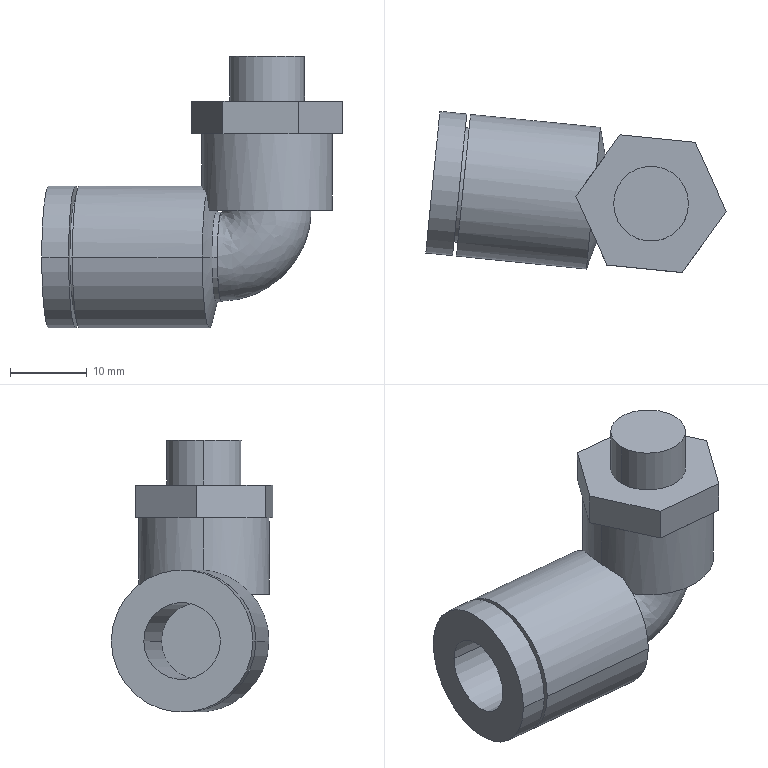Part | SolidWorks | features BaseBody 1 | 1 solid | 38 faces | box 39.045 x 20.983 x 35.35 mm | volume 8720 mm3 | plane 20 | cylinder 14 | cone 2 | spline 2 | commonest cylinder face diameters 18.5 x4 9.728 x2 10 x2 11.729 x2 15 x2 17 x2
STEP:
#1=CARTESIAN_POINT('',(-83.459,11.64,316.618));
#2=VERTEX_POINT('',#1);
#3=CARTESIAN_POINT('',(-85.298,-6.769,316.618));
#4=VERTEX_POINT('',#3);
#5=CARTESIAN_POINT('',(-84.379,2.436,316.618));
#6=DIRECTION('',(0.995,-0.09941,0.));
#7=DIRECTION('',(0.09941,0.995,0.));
#8=AXIS2_PLACEMENT_3D('',#5,#6,#7);
#9=CIRCLE('',#8,9.25);
#10=EDGE_CURVE('',#2,#4,#9,.T.);
#11=ORIENTED_EDGE('',*,*,#10,.T.);
#12=CARTESIAN_POINT('',(-68.414,-8.455,316.618));
#13=VERTEX_POINT('',#12);
#14=CARTESIAN_POINT('',(-76.856,-7.612,316.618));
#15=DIRECTION('',(0.995,-0.09941,0.));
#16=VECTOR('',#15,1000.);
#17=LINE('',#14,#16);
#18=EDGE_CURVE('',#4,#13,#17,.T.);
#19=ORIENTED_EDGE('',*,*,#18,.T.);
#20=CARTESIAN_POINT('',(-67.886,-3.171,324.987));
#21=VERTEX_POINT('',#20);
#22=CARTESIAN_POINT('',(-67.495,0.7488,316.618));
#23=DIRECTION('',(-0.995,0.09941,0.));
#24=DIRECTION('',(0.09941,0.995,0.));
#25=AXIS2_PLACEMENT_3D('',#22,#23,#24);
#26=CIRCLE('',#25,9.25);
#27=EDGE_CURVE('',#13,#21,#26,.T.);
#28=ORIENTED_EDGE('',*,*,#27,.T.);
#29=CARTESIAN_POINT('',(-68.5,0.,325.829));
#30=VERTEX_POINT('',#29);
#31=CARTESIAN_POINT('',(-67.886,-3.171,324.987));
#32=CARTESIAN_POINT('',(-68.081,-2.687,325.205));
#33=CARTESIAN_POINT('',(-68.233,-2.18,325.388));
#34=CARTESIAN_POINT('',(-68.391,-1.383,325.604));
#35=CARTESIAN_POINT('',(-68.432,-1.11,325.666));
#36=CARTESIAN_POINT('',(-68.486,-0.5568,325.766));
#37=CARTESIAN_POINT('',(-68.5,-0.2791,325.804));
#38=CARTESIAN_POINT('',(-68.5,0.,325.829));
#39=B_SPLINE_CURVE_WITH_KNOTS('',3,(#31,#32,#33,#34,#35,#36,#37,#38),.UNSPECIFIED.,.F.,.F.,(4,2,2,4),(-0.004184,-0.002512,-0.001676,-0.0008395),.UNSPECIFIED.);
#40=EDGE_CURVE('',#21,#30,#39,.T.);
#41=ORIENTED_EDGE('',*,*,#40,.T.);
#42=CARTESIAN_POINT('',(-67.103,4.668,324.987));
#43=VERTEX_POINT('',#42);
#44=CARTESIAN_POINT('',(-68.5,0.,325.829));
#45=CARTESIAN_POINT('',(-68.5,0.2097,325.848));
#46=CARTESIAN_POINT('',(-68.492,0.4202,325.86));
#47=CARTESIAN_POINT('',(-68.461,0.8429,325.87));
#48=CARTESIAN_POINT('',(-68.437,1.055,325.868));
#49=CARTESIAN_POINT('',(-68.343,1.68,325.839));
#50=CARTESIAN_POINT('',(-68.251,2.086,325.792));
#51=CARTESIAN_POINT('',(-68.009,2.877,325.643));
#52=CARTESIAN_POINT('',(-67.858,3.265,325.542));
#53=CARTESIAN_POINT('',(-67.513,3.995,325.295));
#54=CARTESIAN_POINT('',(-67.319,4.341,325.151));
#55=CARTESIAN_POINT('',(-67.103,4.668,324.987));
#56=B_SPLINE_CURVE_WITH_KNOTS('',3,(#44,#45,#46,#47,#48,#49,#50,#51,#52,#53,#54,#55),.UNSPECIFIED.,.F.,.F.,(4,2,2,2,2,4),(-0.0008395,-0.0002113,0.000417,0.001674,0.00293,0.004187),.UNSPECIFIED.);
#57=EDGE_CURVE('',#30,#43,#56,.T.);
#58=ORIENTED_EDGE('',*,*,#57,.T.);
#59=CARTESIAN_POINT('',(-66.575,9.953,316.618));
#60=VERTEX_POINT('',#59);
#61=CARTESIAN_POINT('',(-67.495,0.7488,316.618));
#62=DIRECTION('',(-0.995,0.09941,0.));
#63=DIRECTION('',(0.09941,0.995,0.));
#64=AXIS2_PLACEMENT_3D('',#61,#62,#63);
#65=CIRCLE('',#64,9.25);
#66=EDGE_CURVE('',#43,#60,#65,.T.);
#67=ORIENTED_EDGE('',*,*,#66,.T.);
#68=CARTESIAN_POINT('',(-75.017,10.796,316.618));
#69=DIRECTION('',(0.995,-0.09941,0.));
#70=VECTOR('',#69,1000.);
#71=LINE('',#68,#70);
#72=EDGE_CURVE('',#2,#60,#71,.T.);
#73=ORIENTED_EDGE('',*,*,#72,.F.);
#74=EDGE_LOOP('',(#11,#19,#28,#41,#58,#67,#73));
#75=FACE_OUTER_BOUND('',#74,.T.);
#76=CARTESIAN_POINT('',(-75.937,1.592,316.618));
#77=DIRECTION('',(0.995,-0.09941,0.));
#78=DIRECTION('',(0.09941,0.995,0.));
#79=AXIS2_PLACEMENT_3D('',#76,#77,#78);
#80=CYLINDRICAL_SURFACE('',#79,9.25);
#81=ADVANCED_FACE('',(#75),#80,.T.);
#82=CARTESIAN_POINT('',(-67.175,-5.177,316.618));
#83=VERTEX_POINT('',#82);
#84=CARTESIAN_POINT('',(-66.009,6.494,316.618));
#85=VERTEX_POINT('',#84);
#86=CARTESIAN_POINT('',(-66.592,0.6586,316.618));
#87=DIRECTION('',(-0.995,0.09941,0.));
#88=DIRECTION('',(-0.09941,-0.995,0.));
#89=AXIS2_PLACEMENT_3D('',#86,#87,#88);
#90=CIRCLE('',#89,5.864);
#91=EDGE_CURVE('',#83,#85,#90,.T.);
#92=ORIENTED_EDGE('',*,*,#91,.T.);
#93=CARTESIAN_POINT('',(-66.575,9.953,316.618));
#94=DIRECTION('',(-0.1615,0.9869,0.));
#95=VECTOR('',#94,1000.);
#96=LINE('',#93,#95);
#97=EDGE_CURVE('',#85,#60,#96,.T.);
#98=ORIENTED_EDGE('',*,*,#97,.T.);
#99=ORIENTED_EDGE('',*,*,#66,.F.);
#100=CARTESIAN_POINT('',(-66.613,5.34,322.723));
#101=VERTEX_POINT('',#100);
#102=CARTESIAN_POINT('',(-67.103,4.668,324.987));
#103=CARTESIAN_POINT('',(-66.929,4.934,324.247));
#104=CARTESIAN_POINT('',(-66.763,5.154,323.492));
#105=CARTESIAN_POINT('',(-66.613,5.34,322.723));
#106=B_SPLINE_CURVE_WITH_KNOTS('',3,(#102,#103,#104,#105),.UNSPECIFIED.,.F.,.F.,(4,4),(0.,0.002412),.UNSPECIFIED.);
#107=EDGE_CURVE('',#43,#101,#106,.T.);
#108=ORIENTED_EDGE('',*,*,#107,.T.);
#109=CARTESIAN_POINT('',(-67.539,-3.927,322.723));
#110=VERTEX_POINT('',#109);
#111=CARTESIAN_POINT('',(-66.613,5.34,322.723));
#112=CARTESIAN_POINT('',(-66.565,4.561,322.723));
#113=CARTESIAN_POINT('',(-66.536,3.781,322.723));
#114=CARTESIAN_POINT('',(-66.542,2.223,322.723));
#115=CARTESIAN_POINT('',(-66.579,1.444,322.723));
#116=CARTESIAN_POINT('',(-66.734,-0.1136,322.723));
#117=CARTESIAN_POINT('',(-66.853,-0.8843,322.723));
#118=CARTESIAN_POINT('',(-67.155,-2.413,322.723));
#119=CARTESIAN_POINT('',(-67.337,-3.172,322.723));
#120=CARTESIAN_POINT('',(-67.539,-3.927,322.723));
#121=B_SPLINE_CURVE_WITH_KNOTS('',3,(#111,#112,#113,#114,#115,#116,#117,#118,#119,#120),.UNSPECIFIED.,.F.,.F.,(4,2,2,2,4),(0.,0.002338,0.004676,0.007013,0.009351),.UNSPECIFIED.);
#122=EDGE_CURVE('',#101,#110,#121,.T.);
#123=ORIENTED_EDGE('',*,*,#122,.T.);
#124=CARTESIAN_POINT('',(-67.886,-3.171,324.987));
#125=CARTESIAN_POINT('',(-67.768,-3.466,324.247));
#126=CARTESIAN_POINT('',(-67.649,-3.714,323.492));
#127=CARTESIAN_POINT('',(-67.539,-3.927,322.723));
#128=B_SPLINE_CURVE_WITH_KNOTS('',3,(#124,#125,#126,#127),.UNSPECIFIED.,.F.,.F.,(4,4),(0.,0.002412),.UNSPECIFIED.);
#129=EDGE_CURVE('',#21,#110,#128,.T.);
#130=ORIENTED_EDGE('',*,*,#129,.F.);
#131=ORIENTED_EDGE('',*,*,#27,.F.);
#132=CARTESIAN_POINT('',(-68.414,-8.455,316.618));
#133=DIRECTION('',(-0.3536,-0.9354,0.));
#134=VECTOR('',#133,1000.);
#135=LINE('',#132,#134);
#136=EDGE_CURVE('',#83,#13,#135,.T.);
#137=ORIENTED_EDGE('',*,*,#136,.F.);
#138=EDGE_LOOP('',(#92,#98,#99,#108,#123,#130,#131,#137));
#139=FACE_OUTER_BOUND('',#138,.T.);
#140=CARTESIAN_POINT('',(-67.495,0.7488,316.618));
#141=DIRECTION('',(-0.995,0.09941,0.));
#142=DIRECTION('',(-0.09941,-0.995,0.));
#143=AXIS2_PLACEMENT_3D('',#140,#141,#142);
#144=CONICAL_SURFACE('',#143,9.25,1.309);
#145=ADVANCED_FACE('',(#139),#144,.T.);
#146=CARTESIAN_POINT('',(-52.253,3.497,332.631));
#147=VERTEX_POINT('',#146);
#148=CARTESIAN_POINT('',(-51.5,0.,332.631));
#149=VERTEX_POINT('',#148);
#150=CARTESIAN_POINT('',(-60.,0.,332.631));
#151=DIRECTION('',(0.,0.,-1.));
#152=DIRECTION('',(-1.,0.,0.));
#153=AXIS2_PLACEMENT_3D('',#150,#151,#152);
#154=CIRCLE('',#153,8.5);
#155=EDGE_CURVE('',#147,#149,#154,.T.);
#156=ORIENTED_EDGE('',*,*,#155,.T.);
#157=CARTESIAN_POINT('',(-51.5,0.,322.723));
#158=VERTEX_POINT('',#157);
#159=CARTESIAN_POINT('',(-51.5,0.,329.705));
#160=DIRECTION('',(0.,0.,-1.));
#161=VECTOR('',#160,1000.);
#162=LINE('',#159,#161);
#163=EDGE_CURVE('',#149,#158,#162,.T.);
#164=ORIENTED_EDGE('',*,*,#163,.T.);
#165=CARTESIAN_POINT('',(-60.,0.,322.723));
#166=DIRECTION('',(0.,0.,1.));
#167=DIRECTION('',(-1.,0.,0.));
#168=AXIS2_PLACEMENT_3D('',#165,#166,#167);
#169=CIRCLE('',#168,8.5);
#170=EDGE_CURVE('',#158,#101,#169,.T.);
#171=ORIENTED_EDGE('',*,*,#170,.T.);
#172=ORIENTED_EDGE('',*,*,#107,.F.);
#173=ORIENTED_EDGE('',*,*,#57,.F.);
#174=CARTESIAN_POINT('',(-68.5,0.,332.631));
#175=VERTEX_POINT('',#174);
#176=CARTESIAN_POINT('',(-68.5,0.,329.705));
#177=DIRECTION('',(0.,0.,-1.));
#178=VECTOR('',#177,1000.);
#179=LINE('',#176,#178);
#180=EDGE_CURVE('',#175,#30,#179,.T.);
#181=ORIENTED_EDGE('',*,*,#180,.F.);
#182=CARTESIAN_POINT('',(-66.902,4.961,332.631));
#183=VERTEX_POINT('',#182);
#184=CARTESIAN_POINT('',(-60.,0.,332.631));
#185=DIRECTION('',(0.,0.,-1.));
#186=DIRECTION('',(-1.,0.,0.));
#187=AXIS2_PLACEMENT_3D('',#184,#185,#186);
#188=CIRCLE('',#187,8.5);
#189=EDGE_CURVE('',#175,#183,#188,.T.);
#190=ORIENTED_EDGE('',*,*,#189,.T.);
#191=CARTESIAN_POINT('',(-59.155,8.458,332.631));
#192=VERTEX_POINT('',#191);
#193=CARTESIAN_POINT('',(-60.,0.,332.631));
#194=DIRECTION('',(0.,0.,-1.));
#195=DIRECTION('',(-1.,0.,0.));
#196=AXIS2_PLACEMENT_3D('',#193,#194,#195);
#197=CIRCLE('',#196,8.5);
#198=EDGE_CURVE('',#183,#192,#197,.T.);
#199=ORIENTED_EDGE('',*,*,#198,.T.);
#200=CARTESIAN_POINT('',(-60.,0.,332.631));
#201=DIRECTION('',(0.,0.,-1.));
#202=DIRECTION('',(-1.,0.,0.));
#203=AXIS2_PLACEMENT_3D('',#200,#201,#202);
#204=CIRCLE('',#203,8.5);
#205=EDGE_CURVE('',#192,#147,#204,.T.);
#206=ORIENTED_EDGE('',*,*,#205,.T.);
#207=EDGE_LOOP('',(#156,#164,#171,#172,#173,#181,#190,#199,#206));
#208=FACE_OUTER_BOUND('',#207,.T.);
#209=CARTESIAN_POINT('',(-60.,0.,329.705));
#210=DIRECTION('',(0.,0.,-1.));
#211=DIRECTION('',(-1.,0.,0.));
#212=AXIS2_PLACEMENT_3D('',#209,#210,#211);
#213=CYLINDRICAL_SURFACE('',#212,8.5);
#214=ADVANCED_FACE('',(#208),#213,.T.);
#215=ORIENTED_EDGE('',*,*,#91,.F.);
#216=CARTESIAN_POINT('',(-66.474,-5.247,316.618));
#217=VERTEX_POINT('',#216);
#218=CARTESIAN_POINT('',(-66.824,-5.212,316.618));
#219=DIRECTION('',(0.995,-0.09941,0.));
#220=VECTOR('',#219,1000.);
#221=LINE('',#218,#220);
#222=EDGE_CURVE('',#83,#217,#221,.T.);
#223=ORIENTED_EDGE('',*,*,#222,.T.);
#224=CARTESIAN_POINT('',(-65.308,6.424,316.618));
#225=VERTEX_POINT('',#224);
#226=CARTESIAN_POINT('',(-65.891,0.5885,316.618));
#227=DIRECTION('',(-0.995,0.09941,0.));
#228=DIRECTION('',(0.09941,0.995,0.));
#229=AXIS2_PLACEMENT_3D('',#226,#227,#228);
#230=CIRCLE('',#229,5.865);
#231=EDGE_CURVE('',#217,#225,#230,.T.);
#232=ORIENTED_EDGE('',*,*,#231,.T.);
#233=CARTESIAN_POINT('',(-65.658,6.459,316.618));
#234=DIRECTION('',(0.995,-0.09941,0.));
#235=VECTOR('',#234,1000.);
#236=LINE('',#233,#235);
#237=EDGE_CURVE('',#85,#225,#236,.T.);
#238=ORIENTED_EDGE('',*,*,#237,.F.);
#239=EDGE_LOOP('',(#215,#223,#232,#238));
#240=FACE_OUTER_BOUND('',#239,.T.);
#241=CARTESIAN_POINT('',(-66.241,0.6236,316.618));
#242=DIRECTION('',(0.995,-0.09941,0.));
#243=DIRECTION('',(0.09941,0.995,0.));
#244=AXIS2_PLACEMENT_3D('',#241,#242,#243);
#245=CYLINDRICAL_SURFACE('',#244,5.865);
#246=ADVANCED_FACE('',(#240),#245,.T.);
#247=CARTESIAN_POINT('',(-84.131,9.948,316.618));
#248=VERTEX_POINT('',#247);
#249=CARTESIAN_POINT('',(-85.622,-4.978,316.618));
#250=VERTEX_POINT('',#249);
#251=CARTESIAN_POINT('',(-84.876,2.485,316.618));
#252=DIRECTION('',(0.995,-0.09941,0.));
#253=DIRECTION('',(0.09941,0.995,0.));
#254=AXIS2_PLACEMENT_3D('',#251,#252,#253);
#255=CIRCLE('',#254,7.5);
#256=EDGE_CURVE('',#248,#250,#255,.T.);
#257=ORIENTED_EDGE('',*,*,#256,.T.);
#258=CARTESIAN_POINT('',(-85.124,-5.027,316.618));
#259=VERTEX_POINT('',#258);
#260=CARTESIAN_POINT('',(-85.373,-5.002,316.618));
#261=DIRECTION('',(0.995,-0.09941,0.));
#262=VECTOR('',#261,1000.);
#263=LINE('',#260,#262);
#264=EDGE_CURVE('',#250,#259,#263,.T.);
#265=ORIENTED_EDGE('',*,*,#264,.T.);
#266=CARTESIAN_POINT('',(-83.633,9.898,316.618));
#267=VERTEX_POINT('',#266);
#268=CARTESIAN_POINT('',(-84.379,2.436,316.618));
#269=DIRECTION('',(0.995,-0.09941,0.));
#270=DIRECTION('',(0.09941,0.995,0.));
#271=AXIS2_PLACEMENT_3D('',#268,#269,#270);
#272=CIRCLE('',#271,7.5);
#273=EDGE_CURVE('',#267,#259,#272,.T.);
#274=ORIENTED_EDGE('',*,*,#273,.F.);
#275=CARTESIAN_POINT('',(-83.882,9.923,316.618));
#276=DIRECTION('',(0.995,-0.09941,0.));
#277=VECTOR('',#276,1000.);
#278=LINE('',#275,#277);
#279=EDGE_CURVE('',#248,#267,#278,.T.);
#280=ORIENTED_EDGE('',*,*,#279,.F.);
#281=EDGE_LOOP('',(#257,#265,#274,#280));
#282=FACE_OUTER_BOUND('',#281,.T.);
#283=CARTESIAN_POINT('',(-84.627,2.46,316.618));
#284=DIRECTION('',(0.995,-0.09941,0.));
#285=DIRECTION('',(0.09941,0.995,0.));
#286=AXIS2_PLACEMENT_3D('',#283,#284,#285);
#287=CYLINDRICAL_SURFACE('',#286,7.5);
#288=ADVANCED_FACE('',(#282),#287,.T.);
#289=CARTESIAN_POINT('',(-87.439,12.037,316.618));
#290=VERTEX_POINT('',#289);
#291=CARTESIAN_POINT('',(-89.278,-6.371,316.618));
#292=VERTEX_POINT('',#291);
#293=CARTESIAN_POINT('',(-88.359,2.833,316.618));
#294=DIRECTION('',(0.995,-0.09941,0.));
#295=DIRECTION('',(0.09941,0.995,0.));
#296=AXIS2_PLACEMENT_3D('',#293,#294,#295);
#297=CIRCLE('',#296,9.25);
#298=EDGE_CURVE('',#290,#292,#297,.T.);
#299=ORIENTED_EDGE('',*,*,#298,.T.);
#300=CARTESIAN_POINT('',(-85.796,-6.719,316.618));
#301=VERTEX_POINT('',#300);
#302=CARTESIAN_POINT('',(-86.542,-6.644,316.618));
#303=DIRECTION('',(0.995,-0.09941,0.));
#304=VECTOR('',#303,1000.);
#305=LINE('',#302,#304);
#306=EDGE_CURVE('',#292,#301,#305,.T.);
#307=ORIENTED_EDGE('',*,*,#306,.T.);
#308=CARTESIAN_POINT('',(-83.957,11.69,316.618));
#309=VERTEX_POINT('',#308);
#310=CARTESIAN_POINT('',(-84.876,2.485,316.618));
#311=DIRECTION('',(0.995,-0.09941,0.));
#312=DIRECTION('',(0.09941,0.995,0.));
#313=AXIS2_PLACEMENT_3D('',#310,#311,#312);
#314=CIRCLE('',#313,9.25);
#315=EDGE_CURVE('',#309,#301,#314,.T.);
#316=ORIENTED_EDGE('',*,*,#315,.F.);
#317=CARTESIAN_POINT('',(-84.703,11.764,316.618));
#318=DIRECTION('',(0.995,-0.09941,0.));
#319=VECTOR('',#318,1000.);
#320=LINE('',#317,#319);
#321=EDGE_CURVE('',#290,#309,#320,.T.);
#322=ORIENTED_EDGE('',*,*,#321,.F.);
#323=EDGE_LOOP('',(#299,#307,#316,#322));
#324=FACE_OUTER_BOUND('',#323,.T.);
#325=CARTESIAN_POINT('',(-85.622,2.56,316.618));
#326=DIRECTION('',(0.995,-0.09941,0.));
#327=DIRECTION('',(0.09941,0.995,0.));
#328=AXIS2_PLACEMENT_3D('',#325,#326,#327);
#329=CYLINDRICAL_SURFACE('',#328,9.25);
#330=ADVANCED_FACE('',(#324),#329,.T.);
#331=CARTESIAN_POINT('',(-64.864,0.,342.718));
#332=VERTEX_POINT('',#331);
#333=CARTESIAN_POINT('',(-55.136,0.,342.718));
#334=VERTEX_POINT('',#333);
#335=CARTESIAN_POINT('',(-60.,0.,342.718));
#336=DIRECTION('',(0.,0.,-1.));
#337=DIRECTION('',(-1.,0.,0.));
#338=AXIS2_PLACEMENT_3D('',#335,#336,#337);
#339=CIRCLE('',#338,4.864);
#340=EDGE_CURVE('',#332,#334,#339,.T.);
#341=ORIENTED_EDGE('',*,*,#340,.T.);
#342=CARTESIAN_POINT('',(-55.136,0.,336.881));
#343=VERTEX_POINT('',#342);
#344=CARTESIAN_POINT('',(-55.136,0.,339.702));
#345=DIRECTION('',(0.,0.,-1.));
#346=VECTOR('',#345,1000.);
#347=LINE('',#344,#346);
#348=EDGE_CURVE('',#334,#343,#347,.T.);
#349=ORIENTED_EDGE('',*,*,#348,.T.);
#350=CARTESIAN_POINT('',(-64.864,0.,336.881));
#351=VERTEX_POINT('',#350);
#352=CARTESIAN_POINT('',(-60.,0.,336.881));
#353=DIRECTION('',(0.,0.,1.));
#354=DIRECTION('',(-1.,0.,0.));
#355=AXIS2_PLACEMENT_3D('',#352,#353,#354);
#356=CIRCLE('',#355,4.864);
#357=EDGE_CURVE('',#343,#351,#356,.T.);
#358=ORIENTED_EDGE('',*,*,#357,.T.);
#359=CARTESIAN_POINT('',(-64.864,0.,339.702));
#360=DIRECTION('',(0.,0.,-1.));
#361=VECTOR('',#360,1000.);
#362=LINE('',#359,#361);
#363=EDGE_CURVE('',#332,#351,#362,.T.);
#364=ORIENTED_EDGE('',*,*,#363,.F.);
#365=EDGE_LOOP('',(#341,#349,#358,#364));
#366=FACE_OUTER_BOUND('',#365,.T.);
#367=CARTESIAN_POINT('',(-60.,0.,339.702));
#368=DIRECTION('',(0.,0.,-1.));
#369=DIRECTION('',(-1.,0.,0.));
#370=AXIS2_PLACEMENT_3D('',#367,#368,#369);
#371=CYLINDRICAL_SURFACE('',#370,4.864);
#372=ADVANCED_FACE('',(#366),#371,.T.);
#373=CARTESIAN_POINT('',(-64.976,5.522,316.618));
#374=VERTEX_POINT('',#373);
#375=CARTESIAN_POINT('',(-65.97,-4.428,316.618));
#376=VERTEX_POINT('',#375);
#377=CARTESIAN_POINT('',(-65.473,0.5468,316.618));
#378=DIRECTION('',(-0.995,0.09941,0.));
#379=DIRECTION('',(-0.09941,-0.995,0.));
#380=AXIS2_PLACEMENT_3D('',#377,#378,#379);
#381=CIRCLE('',#380,5.);
#382=EDGE_CURVE('',#374,#376,#381,.T.);
#383=ORIENTED_EDGE('',*,*,#382,.F.);
#384=CARTESIAN_POINT('',(-87.862,7.809,316.618));
#385=VERTEX_POINT('',#384);
#386=CARTESIAN_POINT('',(-106.768,9.697,316.618));
#387=DIRECTION('',(-0.995,0.09941,0.));
#388=VECTOR('',#387,1000.);
#389=LINE('',#386,#388);
#390=EDGE_CURVE('',#374,#385,#389,.T.);
#391=ORIENTED_EDGE('',*,*,#390,.T.);
#392=CARTESIAN_POINT('',(-88.856,-2.142,316.618));
#393=VERTEX_POINT('',#392);
#394=CARTESIAN_POINT('',(-88.359,2.833,316.618));
#395=DIRECTION('',(0.995,-0.09941,0.));
#396=DIRECTION('',(-0.09941,-0.995,0.));
#397=AXIS2_PLACEMENT_3D('',#394,#395,#396);
#398=CIRCLE('',#397,5.);
#399=EDGE_CURVE('',#393,#385,#398,.T.);
#400=ORIENTED_EDGE('',*,*,#399,.F.);
#401=CARTESIAN_POINT('',(-107.762,-0.2531,316.618));
#402=DIRECTION('',(-0.995,0.09941,0.));
#403=VECTOR('',#402,1000.);
#404=LINE('',#401,#403);
#405=EDGE_CURVE('',#376,#393,#404,.T.);
#406=ORIENTED_EDGE('',*,*,#405,.F.);
#407=EDGE_LOOP('',(#383,#391,#400,#406));
#408=FACE_OUTER_BOUND('',#407,.T.);
#409=CARTESIAN_POINT('',(-107.265,4.722,316.618));
#410=DIRECTION('',(-0.995,0.09941,0.));
#411=DIRECTION('',(-0.09941,-0.995,0.));
#412=AXIS2_PLACEMENT_3D('',#409,#410,#411);
#413=CYLINDRICAL_SURFACE('',#412,5.);
#414=ADVANCED_FACE('',(#408),#413,.F.);
#415=ORIENTED_EDGE('',*,*,#18,.F.);
#416=CARTESIAN_POINT('',(-84.379,2.436,316.618));
#417=DIRECTION('',(0.995,-0.09941,0.));
#418=DIRECTION('',(0.09941,0.995,0.));
#419=AXIS2_PLACEMENT_3D('',#416,#417,#418);
#420=CIRCLE('',#419,9.25);
#421=EDGE_CURVE('',#4,#2,#420,.T.);
#422=ORIENTED_EDGE('',*,*,#421,.T.);
#423=ORIENTED_EDGE('',*,*,#72,.T.);
#424=CARTESIAN_POINT('',(-67.495,0.7488,316.618));
#425=DIRECTION('',(-0.995,0.09941,0.));
#426=DIRECTION('',(0.09941,0.995,0.));
#427=AXIS2_PLACEMENT_3D('',#424,#425,#426);
#428=CIRCLE('',#427,9.25);
#429=EDGE_CURVE('',#60,#13,#428,.T.);
#430=ORIENTED_EDGE('',*,*,#429,.T.);
#431=EDGE_LOOP('',(#415,#422,#423,#430));
#432=FACE_OUTER_BOUND('',#431,.T.);
#433=CARTESIAN_POINT('',(-75.937,1.592,316.618));
#434=DIRECTION('',(0.995,-0.09941,0.));
#435=DIRECTION('',(0.09941,0.995,0.));
#436=AXIS2_PLACEMENT_3D('',#433,#434,#435);
#437=CYLINDRICAL_SURFACE('',#436,9.25);
#438=ADVANCED_FACE('',(#432),#437,.T.);
#439=ORIENTED_EDGE('',*,*,#97,.F.);
#440=CARTESIAN_POINT('',(-66.592,0.6586,316.618));
#441=DIRECTION('',(-0.995,0.09941,0.));
#442=DIRECTION('',(-0.09941,-0.995,0.));
#443=AXIS2_PLACEMENT_3D('',#440,#441,#442);
#444=CIRCLE('',#443,5.864);
#445=EDGE_CURVE('',#85,#83,#444,.T.);
#446=ORIENTED_EDGE('',*,*,#445,.T.);
#447=ORIENTED_EDGE('',*,*,#136,.T.);
#448=ORIENTED_EDGE('',*,*,#429,.F.);
#449=EDGE_LOOP('',(#439,#446,#447,#448));
#450=FACE_OUTER_BOUND('',#449,.T.);
#451=CARTESIAN_POINT('',(-67.495,0.7488,316.618));
#452=DIRECTION('',(-0.995,0.09941,0.));
#453=DIRECTION('',(-0.09941,-0.995,0.));
#454=AXIS2_PLACEMENT_3D('',#451,#452,#453);
#455=CONICAL_SURFACE('',#454,9.25,1.309);
#456=ADVANCED_FACE('',(#450),#455,.T.);
#457=ORIENTED_EDGE('',*,*,#163,.F.);
#458=CARTESIAN_POINT('',(-53.098,-4.961,332.631));
#459=VERTEX_POINT('',#458);
#460=CARTESIAN_POINT('',(-60.,0.,332.631));
#461=DIRECTION('',(0.,0.,-1.));
#462=DIRECTION('',(-1.,0.,0.));
#463=AXIS2_PLACEMENT_3D('',#460,#461,#462);
#464=CIRCLE('',#463,8.5);
#465=EDGE_CURVE('',#149,#459,#464,.T.);
#466=ORIENTED_EDGE('',*,*,#465,.T.);
#467=CARTESIAN_POINT('',(-60.845,-8.458,332.631));
#468=VERTEX_POINT('',#467);
#469=CARTESIAN_POINT('',(-60.,0.,332.631));
#470=DIRECTION('',(0.,0.,-1.));
#471=DIRECTION('',(-1.,0.,0.));
#472=AXIS2_PLACEMENT_3D('',#469,#470,#471);
#473=CIRCLE('',#472,8.5);
#474=EDGE_CURVE('',#459,#468,#473,.T.);
#475=ORIENTED_EDGE('',*,*,#474,.T.);
#476=CARTESIAN_POINT('',(-67.747,-3.497,332.631));
#477=VERTEX_POINT('',#476);
#478=CARTESIAN_POINT('',(-60.,0.,332.631));
#479=DIRECTION('',(0.,0.,-1.));
#480=DIRECTION('',(-1.,0.,0.));
#481=AXIS2_PLACEMENT_3D('',#478,#479,#480);
#482=CIRCLE('',#481,8.5);
#483=EDGE_CURVE('',#468,#477,#482,.T.);
#484=ORIENTED_EDGE('',*,*,#483,.T.);
#485=CARTESIAN_POINT('',(-60.,0.,332.631));
#486=DIRECTION('',(0.,0.,-1.));
#487=DIRECTION('',(-1.,0.,0.));
#488=AXIS2_PLACEMENT_3D('',#485,#486,#487);
#489=CIRCLE('',#488,8.5);
#490=EDGE_CURVE('',#477,#175,#489,.T.);
#491=ORIENTED_EDGE('',*,*,#490,.T.);
#492=ORIENTED_EDGE('',*,*,#180,.T.);
#493=ORIENTED_EDGE('',*,*,#40,.F.);
#494=ORIENTED_EDGE('',*,*,#129,.T.);
#495=CARTESIAN_POINT('',(-60.,0.,322.723));
#496=DIRECTION('',(0.,0.,1.));
#497=DIRECTION('',(-1.,0.,0.));
#498=AXIS2_PLACEMENT_3D('',#495,#496,#497);
#499=CIRCLE('',#498,8.5);
#500=EDGE_CURVE('',#110,#158,#499,.T.);
#501=ORIENTED_EDGE('',*,*,#500,.T.);
#502=EDGE_LOOP('',(#457,#466,#475,#484,#491,#492,#493,#494,#501));
#503=FACE_OUTER_BOUND('',#502,.T.);
#504=CARTESIAN_POINT('',(-60.,0.,329.705));
#505=DIRECTION('',(0.,0.,-1.));
#506=DIRECTION('',(-1.,0.,0.));
#507=AXIS2_PLACEMENT_3D('',#504,#505,#506);
#508=CYLINDRICAL_SURFACE('',#507,8.5);
#509=ADVANCED_FACE('',(#503),#508,.T.);
#510=ORIENTED_EDGE('',*,*,#273,.T.);
#511=CARTESIAN_POINT('',(-84.379,2.436,316.618));
#512=DIRECTION('',(0.995,-0.09941,0.));
#513=DIRECTION('',(0.09941,0.995,0.));
#514=AXIS2_PLACEMENT_3D('',#511,#512,#513);
#515=CIRCLE('',#514,7.5);
#516=EDGE_CURVE('',#259,#267,#515,.T.);
#517=ORIENTED_EDGE('',*,*,#516,.T.);
#518=EDGE_LOOP('',(#510,#517));
#519=FACE_BOUND('',#518,.T.);
#520=ORIENTED_EDGE('',*,*,#10,.F.);
#521=ORIENTED_EDGE('',*,*,#421,.F.);
#522=EDGE_LOOP('',(#520,#521));
#523=FACE_OUTER_BOUND('',#522,.T.);
#524=CARTESIAN_POINT('',(-85.211,-5.898,316.618));
#525=DIRECTION('',(-0.995,0.09941,0.));
#526=DIRECTION('',(-0.09941,-0.995,0.));
#527=AXIS2_PLACEMENT_3D('',#524,#525,#526);
#528=PLANE('',#527);
#529=ADVANCED_FACE('',(#519,#523),#528,.T.);
#530=ORIENTED_EDGE('',*,*,#222,.F.);
#531=ORIENTED_EDGE('',*,*,#445,.F.);
#532=ORIENTED_EDGE('',*,*,#237,.T.);
#533=CARTESIAN_POINT('',(-65.891,0.5885,316.618));
#534=DIRECTION('',(-0.995,0.09941,0.));
#535=DIRECTION('',(0.09941,0.995,0.));
#536=AXIS2_PLACEMENT_3D('',#533,#534,#535);
#537=CIRCLE('',#536,5.865);
#538=EDGE_CURVE('',#225,#217,#537,.T.);
#539=ORIENTED_EDGE('',*,*,#538,.T.);
#540=EDGE_LOOP('',(#530,#531,#532,#539));
#541=FACE_OUTER_BOUND('',#540,.T.);
#542=CARTESIAN_POINT('',(-66.241,0.6236,316.618));
#543=DIRECTION('',(0.995,-0.09941,0.));
#544=DIRECTION('',(0.09941,0.995,0.));
#545=AXIS2_PLACEMENT_3D('',#542,#543,#544);
#546=CYLINDRICAL_SURFACE('',#545,5.865);
#547=ADVANCED_FACE('',(#541),#546,.T.);
#548=ORIENTED_EDGE('',*,*,#122,.F.);
#549=ORIENTED_EDGE('',*,*,#170,.F.);
#550=ORIENTED_EDGE('',*,*,#500,.F.);
#551=EDGE_LOOP('',(#548,#549,#550));
#552=FACE_OUTER_BOUND('',#551,.T.);
#553=CARTESIAN_POINT('',(-54.293,-0.5701,322.723));
#554=VERTEX_POINT('',#553);
#555=CARTESIAN_POINT('',(-65.707,0.5701,322.723));
#556=VERTEX_POINT('',#555);
#557=CARTESIAN_POINT('',(-54.293,-0.5701,322.723));
#558=CARTESIAN_POINT('',(-53.153,10.843,322.723));
#559=CARTESIAN_POINT('',(-64.566,11.983,322.723));
#560=CARTESIAN_POINT('',(-65.707,0.5701,322.723));
#561=(BOUNDED_CURVE()B_SPLINE_CURVE(3,(#557,#558,#559,#560),.UNSPECIFIED.,.F.,.T.)B_SPLINE_CURVE_WITH_KNOTS((4,4),(0.,0.01793),.UNSPECIFIED.)CURVE()GEOMETRIC_REPRESENTATION_ITEM()RATIONAL_B_SPLINE_CURVE((1.,0.3333,0.3333,1.))REPRESENTATION_ITEM(''));
#562=EDGE_CURVE('',#554,#556,#561,.T.);
#563=ORIENTED_EDGE('',*,*,#562,.T.);
#564=CARTESIAN_POINT('',(-65.707,0.5701,322.723));
#565=CARTESIAN_POINT('',(-66.847,-10.843,322.723));
#566=CARTESIAN_POINT('',(-55.434,-11.983,322.723));
#567=CARTESIAN_POINT('',(-54.293,-0.5701,322.723));
#568=(BOUNDED_CURVE()B_SPLINE_CURVE(3,(#564,#565,#566,#567),.UNSPECIFIED.,.F.,.T.)B_SPLINE_CURVE_WITH_KNOTS((4,4),(0.,0.01814),.UNSPECIFIED.)CURVE()GEOMETRIC_REPRESENTATION_ITEM()RATIONAL_B_SPLINE_CURVE((1.,0.3333,0.3333,1.))REPRESENTATION_ITEM(''));
#569=EDGE_CURVE('',#556,#554,#568,.T.);
#570=ORIENTED_EDGE('',*,*,#569,.T.);
#571=EDGE_LOOP('',(#563,#570));
#572=FACE_BOUND('',#571,.T.);
#573=CARTESIAN_POINT('',(-60.423,-4.229,322.723));
#574=DIRECTION('',(0.,0.,-1.));
#575=DIRECTION('',(-1.,0.,0.));
#576=AXIS2_PLACEMENT_3D('',#573,#574,#575);
#577=PLANE('',#576);
#578=ADVANCED_FACE('',(#552,#572),#577,.T.);
#579=CARTESIAN_POINT('',(-64.038,8.946,332.631));
#580=VERTEX_POINT('',#579);
#581=CARTESIAN_POINT('',(-64.038,8.946,332.631));
#582=DIRECTION('',(0.995,-0.09941,0.));
#583=VECTOR('',#582,1000.);
#584=LINE('',#581,#583);
#585=EDGE_CURVE('',#580,#192,#584,.T.);
#586=ORIENTED_EDGE('',*,*,#585,.T.);
#587=ORIENTED_EDGE('',*,*,#198,.F.);
#588=CARTESIAN_POINT('',(-66.902,4.961,332.631));
#589=DIRECTION('',(0.5836,0.812,0.));
#590=VECTOR('',#589,1000.);
#591=LINE('',#588,#590);
#592=EDGE_CURVE('',#183,#580,#591,.T.);
#593=ORIENTED_EDGE('',*,*,#592,.T.);
#594=EDGE_LOOP('',(#586,#587,#593));
#595=FACE_OUTER_BOUND('',#594,.T.);
#596=CARTESIAN_POINT('',(-60.,0.,332.631));
#597=DIRECTION('',(0.,0.,-1.));
#598=DIRECTION('',(-1.,0.,0.));
#599=AXIS2_PLACEMENT_3D('',#596,#597,#598);
#600=PLANE('',#599);
#601=ADVANCED_FACE('',(#595),#600,.T.);
#602=CARTESIAN_POINT('',(-69.766,0.9757,332.631));
#603=VERTEX_POINT('',#602);
#604=CARTESIAN_POINT('',(-69.766,0.9757,332.631));
#605=DIRECTION('',(0.5836,0.812,0.));
#606=VECTOR('',#605,1000.);
#607=LINE('',#604,#606);
#608=EDGE_CURVE('',#603,#183,#607,.T.);
#609=ORIENTED_EDGE('',*,*,#608,.T.);
#610=ORIENTED_EDGE('',*,*,#189,.F.);
#611=ORIENTED_EDGE('',*,*,#490,.F.);
#612=CARTESIAN_POINT('',(-67.747,-3.497,332.631));
#613=DIRECTION('',(-0.4114,0.9114,0.));
#614=VECTOR('',#613,1000.);
#615=LINE('',#612,#614);
#616=EDGE_CURVE('',#477,#603,#615,.T.);
#617=ORIENTED_EDGE('',*,*,#616,.T.);
#618=EDGE_LOOP('',(#609,#610,#611,#617));
#619=FACE_OUTER_BOUND('',#618,.T.);
#620=CARTESIAN_POINT('',(-60.,0.,332.631));
#621=DIRECTION('',(0.,0.,-1.));
#622=DIRECTION('',(-1.,0.,0.));
#623=AXIS2_PLACEMENT_3D('',#620,#621,#622);
#624=PLANE('',#623);
#625=ADVANCED_FACE('',(#619),#624,.T.);
#626=CARTESIAN_POINT('',(-65.728,-7.97,332.631));
#627=VERTEX_POINT('',#626);
#628=CARTESIAN_POINT('',(-65.728,-7.97,332.631));
#629=DIRECTION('',(-0.4114,0.9114,0.));
#630=VECTOR('',#629,1000.);
#631=LINE('',#628,#630);
#632=EDGE_CURVE('',#627,#477,#631,.T.);
#633=ORIENTED_EDGE('',*,*,#632,.T.);
#634=ORIENTED_EDGE('',*,*,#483,.F.);
#635=CARTESIAN_POINT('',(-60.845,-8.458,332.631));
#636=DIRECTION('',(-0.995,0.09941,0.));
#637=VECTOR('',#636,1000.);
#638=LINE('',#635,#637);
#639=EDGE_CURVE('',#468,#627,#638,.T.);
#640=ORIENTED_EDGE('',*,*,#639,.T.);
#641=EDGE_LOOP('',(#633,#634,#640));
#642=FACE_OUTER_BOUND('',#641,.T.);
#643=CARTESIAN_POINT('',(-60.,0.,332.631));
#644=DIRECTION('',(0.,0.,-1.));
#645=DIRECTION('',(-1.,0.,0.));
#646=AXIS2_PLACEMENT_3D('',#643,#644,#645);
#647=PLANE('',#646);
#648=ADVANCED_FACE('',(#642),#647,.T.);
#649=ORIENTED_EDGE('',*,*,#264,.F.);
#650=CARTESIAN_POINT('',(-84.876,2.485,316.618));
#651=DIRECTION('',(0.995,-0.09941,0.));
#652=DIRECTION('',(0.09941,0.995,0.));
#653=AXIS2_PLACEMENT_3D('',#650,#651,#652);
#654=CIRCLE('',#653,7.5);
#655=EDGE_CURVE('',#250,#248,#654,.T.);
#656=ORIENTED_EDGE('',*,*,#655,.T.);
#657=ORIENTED_EDGE('',*,*,#279,.T.);
#658=ORIENTED_EDGE('',*,*,#516,.F.);
#659=EDGE_LOOP('',(#649,#656,#657,#658));
#660=FACE_OUTER_BOUND('',#659,.T.);
#661=CARTESIAN_POINT('',(-84.627,2.46,316.618));
#662=DIRECTION('',(0.995,-0.09941,0.));
#663=DIRECTION('',(0.09941,0.995,0.));
#664=AXIS2_PLACEMENT_3D('',#661,#662,#663);
#665=CYLINDRICAL_SURFACE('',#664,7.5);
#666=ADVANCED_FACE('',(#660),#665,.T.);
#667=ORIENTED_EDGE('',*,*,#538,.F.);
#668=ORIENTED_EDGE('',*,*,#231,.F.);
#669=EDGE_LOOP('',(#667,#668));
#670=FACE_OUTER_BOUND('',#669,.T.);
#671=CARTESIAN_POINT('',(-65.891,0.5885,310.884));
#672=VERTEX_POINT('',#671);
#673=CARTESIAN_POINT('',(-65.891,0.5885,322.402));
#674=VERTEX_POINT('',#673);
#675=CARTESIAN_POINT('',(-65.891,0.5885,310.884));
#676=CARTESIAN_POINT('',(-65.928,0.2112,310.884));
#677=CARTESIAN_POINT('',(-65.966,-0.1665,310.922));
#678=CARTESIAN_POINT('',(-66.039,-0.8995,311.07));
#679=CARTESIAN_POINT('',(-66.075,-1.255,311.179));
#680=CARTESIAN_POINT('',(-66.144,-1.945,311.467));
#681=CARTESIAN_POINT('',(-66.177,-2.28,311.648));
#682=CARTESIAN_POINT('',(-66.239,-2.899,312.064));
#683=CARTESIAN_POINT('',(-66.268,-3.186,312.302));
#684=CARTESIAN_POINT('',(-66.321,-3.718,312.837));
#685=CARTESIAN_POINT('',(-66.345,-3.955,313.13));
#686=CARTESIAN_POINT('',(-66.376,-4.264,313.596));
#687=CARTESIAN_POINT('',(-66.385,-4.36,313.757));
#688=CARTESIAN_POINT('',(-66.403,-4.536,314.089));
#689=CARTESIAN_POINT('',(-66.411,-4.616,314.261));
#690=CARTESIAN_POINT('',(-66.432,-4.831,314.784));
#691=CARTESIAN_POINT('',(-66.443,-4.938,315.142));
#692=CARTESIAN_POINT('',(-66.457,-5.082,315.877));
#693=CARTESIAN_POINT('',(-66.461,-5.119,316.257));
#694=CARTESIAN_POINT('',(-66.461,-5.117,317.007));
#695=CARTESIAN_POINT('',(-66.457,-5.08,317.379));
#696=CARTESIAN_POINT('',(-66.446,-4.97,317.933));
#697=CARTESIAN_POINT('',(-66.441,-4.924,318.118));
#698=CARTESIAN_POINT('',(-66.43,-4.814,318.478));
#699=CARTESIAN_POINT('',(-66.424,-4.751,318.654));
#700=CARTESIAN_POINT('',(-66.403,-4.537,319.172));
#701=CARTESIAN_POINT('',(-66.385,-4.361,319.503));
#702=CARTESIAN_POINT('',(-66.343,-3.942,320.132));
#703=CARTESIAN_POINT('',(-66.32,-3.705,320.422));
#704=CARTESIAN_POINT('',(-66.28,-3.31,320.819));
#705=CARTESIAN_POINT('',(-66.266,-3.172,320.945));
#706=CARTESIAN_POINT('',(-66.237,-2.883,321.185));
#707=CARTESIAN_POINT('',(-66.222,-2.731,321.298));
#708=CARTESIAN_POINT('',(-66.176,-2.265,321.613));
#709=CARTESIAN_POINT('',(-66.143,-1.938,321.791));
#710=CARTESIAN_POINT('',(-66.074,-1.251,322.085));
#711=CARTESIAN_POINT('',(-66.038,-0.889,322.201));
#712=CARTESIAN_POINT('',(-65.965,-0.1599,322.359));
#713=CARTESIAN_POINT('',(-65.928,0.2106,322.402));
#714=CARTESIAN_POINT('',(-65.891,0.5885,322.402));
#715=B_SPLINE_CURVE_WITH_KNOTS('',3,(#675,#676,#677,#678,#679,#680,#681,#682,#683,#684,#685,#686,#687,#688,#689,#690,#691,#692,#693,#694,#695,#696,#697,#698,#699,#700,#701,#702,#703,#704,#705,#706,#707,#708,#709,#710,#711,#712,#713,#714),.UNSPECIFIED.,.F.,.F.,(4,2,2,2,2,2,2,2,2,2,2,2,2,2,2,2,2,2,2,4),(0.,0.001135,0.00227,0.003405,0.004541,0.005676,0.006243,0.006811,0.007946,0.009081,0.01022,0.01078,0.01135,0.01249,0.01362,0.01419,0.01476,0.01589,0.01703,0.01816),.UNSPECIFIED.);
#716=EDGE_CURVE('',#672,#674,#715,.T.);
#717=ORIENTED_EDGE('',*,*,#716,.T.);
#718=CARTESIAN_POINT('',(-65.891,0.5885,322.402));
#719=CARTESIAN_POINT('',(-65.853,0.966,322.402));
#720=CARTESIAN_POINT('',(-65.815,1.343,322.358));
#721=CARTESIAN_POINT('',(-65.742,2.074,322.199));
#722=CARTESIAN_POINT('',(-65.707,2.428,322.085));
#723=CARTESIAN_POINT('',(-65.638,3.115,321.791));
#724=CARTESIAN_POINT('',(-65.605,3.449,321.609));
#725=CARTESIAN_POINT('',(-65.543,4.067,321.19));
#726=CARTESIAN_POINT('',(-65.514,4.354,320.953));
#727=CARTESIAN_POINT('',(-65.475,4.752,320.552));
#728=CARTESIAN_POINT('',(-65.462,4.879,320.411));
#729=CARTESIAN_POINT('',(-65.438,5.116,320.121));
#730=CARTESIAN_POINT('',(-65.427,5.227,319.97));
#731=CARTESIAN_POINT('',(-65.396,5.536,319.505));
#732=CARTESIAN_POINT('',(-65.379,5.714,319.173));
#733=CARTESIAN_POINT('',(-65.35,6.002,318.474));
#734=CARTESIAN_POINT('',(-65.339,6.111,318.116));
#735=CARTESIAN_POINT('',(-65.328,6.22,317.566));
#736=CARTESIAN_POINT('',(-65.325,6.248,317.38));
#737=CARTESIAN_POINT('',(-65.322,6.285,317.005));
#738=CARTESIAN_POINT('',(-65.321,6.295,316.815));
#739=CARTESIAN_POINT('',(-65.32,6.296,316.251));
#740=CARTESIAN_POINT('',(-65.324,6.26,315.879));
#741=CARTESIAN_POINT('',(-65.339,6.115,315.142));
#742=CARTESIAN_POINT('',(-65.349,6.005,314.777));
#743=CARTESIAN_POINT('',(-65.378,5.721,314.085));
#744=CARTESIAN_POINT('',(-65.395,5.546,313.755));
#745=CARTESIAN_POINT('',(-65.437,5.129,313.125));
#746=CARTESIAN_POINT('',(-65.461,4.891,312.834));
#747=CARTESIAN_POINT('',(-65.5,4.497,312.437));
#748=CARTESIAN_POINT('',(-65.514,4.359,312.311));
#749=CARTESIAN_POINT('',(-65.543,4.071,312.072));
#750=CARTESIAN_POINT('',(-65.558,3.919,311.958));
#751=CARTESIAN_POINT('',(-65.605,3.451,311.644));
#752=CARTESIAN_POINT('',(-65.637,3.123,311.467));
#753=CARTESIAN_POINT('',(-65.706,2.435,311.18));
#754=CARTESIAN_POINT('',(-65.743,2.071,311.068));
#755=CARTESIAN_POINT('',(-65.816,1.338,310.922));
#756=CARTESIAN_POINT('',(-65.853,0.9658,310.884));
#757=CARTESIAN_POINT('',(-65.891,0.5885,310.884));
#758=B_SPLINE_CURVE_WITH_KNOTS('',3,(#718,#719,#720,#721,#722,#723,#724,#725,#726,#727,#728,#729,#730,#731,#732,#733,#734,#735,#736,#737,#738,#739,#740,#741,#742,#743,#744,#745,#746,#747,#748,#749,#750,#751,#752,#753,#754,#755,#756,#757),.UNSPECIFIED.,.F.,.F.,(4,2,2,2,2,2,2,2,2,2,2,2,2,2,2,2,2,2,2,4),(0.,0.001135,0.00227,0.003405,0.00454,0.005107,0.005675,0.00681,0.007945,0.008512,0.00908,0.01021,0.01135,0.01248,0.01362,0.01419,0.01475,0.01589,0.01702,0.01816),.UNSPECIFIED.);
#759=EDGE_CURVE('',#674,#672,#758,.T.);
#760=ORIENTED_EDGE('',*,*,#759,.T.);
#761=EDGE_LOOP('',(#717,#760));
#762=FACE_BOUND('',#761,.T.);
#763=CARTESIAN_POINT('',(-66.182,-2.329,316.618));
#764=DIRECTION('',(0.995,-0.09941,0.));
#765=DIRECTION('',(0.09941,0.995,0.));
#766=AXIS2_PLACEMENT_3D('',#763,#764,#765);
#767=PLANE('',#766);
#768=ADVANCED_FACE('',(#670,#762),#767,.T.);
#769=CARTESIAN_POINT('',(-65.891,0.5885,310.884));
#770=CARTESIAN_POINT('',(-59.07,-0.09292,310.991));
#771=CARTESIAN_POINT('',(-54.293,-0.5701,315.878));
#772=CARTESIAN_POINT('',(-54.293,-0.5701,322.723));
#773=(BOUNDED_CURVE()B_SPLINE_CURVE(3,(#769,#770,#771,#772),.UNSPECIFIED.,.F.,.T.)B_SPLINE_CURVE_WITH_KNOTS((4,4),(0.006606,1.),.UNSPECIFIED.)CURVE()GEOMETRIC_REPRESENTATION_ITEM()RATIONAL_B_SPLINE_CURVE((0.9962,0.8062,0.8075,1.))REPRESENTATION_ITEM(''));
#774=EDGE_CURVE('',#672,#554,#773,.T.);
#775=ORIENTED_EDGE('',*,*,#774,.T.);
#776=ORIENTED_EDGE('',*,*,#569,.F.);
#777=CARTESIAN_POINT('',(-65.707,0.5701,322.723));
#778=CARTESIAN_POINT('',(-65.707,0.5701,322.591));
#779=CARTESIAN_POINT('',(-65.771,0.5766,322.472));
#780=CARTESIAN_POINT('',(-65.891,0.5885,322.402));
#781=(BOUNDED_CURVE()B_SPLINE_CURVE(3,(#777,#778,#779,#780),.UNSPECIFIED.,.F.,.F.)B_SPLINE_CURVE_WITH_KNOTS((4,4),(0.001639,0.6632),.UNSPECIFIED.)CURVE()GEOMETRIC_REPRESENTATION_ITEM()RATIONAL_B_SPLINE_CURVE((1.,0.8718,0.8284,0.8698))REPRESENTATION_ITEM(''));
#782=EDGE_CURVE('',#556,#674,#781,.T.);
#783=ORIENTED_EDGE('',*,*,#782,.T.);
#784=ORIENTED_EDGE('',*,*,#716,.F.);
#785=EDGE_LOOP('',(#775,#776,#783,#784));
#786=FACE_OUTER_BOUND('',#785,.T.);
#787=CARTESIAN_POINT('',(-66.072,0.6066,322.353));
#788=CARTESIAN_POINT('',(-65.857,0.5852,322.355));
#789=CARTESIAN_POINT('',(-65.707,0.5701,322.508));
#790=CARTESIAN_POINT('',(-65.707,0.5701,322.723));
#791=CARTESIAN_POINT('',(-67.212,-10.807,322.353));
#792=CARTESIAN_POINT('',(-66.998,-10.828,322.355));
#793=CARTESIAN_POINT('',(-66.847,-10.843,322.508));
#794=CARTESIAN_POINT('',(-66.847,-10.843,322.723));
#795=CARTESIAN_POINT('',(-67.114,-10.816,310.883));
#796=CARTESIAN_POINT('',(-60.258,-11.501,310.943));
#797=CARTESIAN_POINT('',(-55.434,-11.983,315.836));
#798=CARTESIAN_POINT('',(-55.434,-11.983,322.723));
#799=CARTESIAN_POINT('',(-65.973,0.5968,310.883));
#800=CARTESIAN_POINT('',(-59.118,-0.08813,310.943));
#801=CARTESIAN_POINT('',(-54.293,-0.5701,315.836));
#802=CARTESIAN_POINT('',(-54.293,-0.5701,322.723));
#803=(BOUNDED_SURFACE()B_SPLINE_SURFACE(3,3,((#787,#788,#789,#790),(#791,#792,#793,#794),(#795,#796,#797,#798),(#799,#800,#801,#802)),.UNSPECIFIED.,.F.,.F.,.F.)B_SPLINE_SURFACE_WITH_KNOTS((4,4),(4,4),(0.,1.),(0.001639,1.),.UNSPECIFIED.)GEOMETRIC_REPRESENTATION_ITEM()RATIONAL_B_SPLINE_SURFACE(((0.999,0.8062,0.8065,1.),(0.333,0.2687,0.2688,0.3333),(0.333,0.2687,0.2688,0.3333),(0.999,0.8062,0.8065,1.)))REPRESENTATION_ITEM('')SURFACE());
#804=ADVANCED_FACE('',(#786),#803,.T.);
#805=ORIENTED_EDGE('',*,*,#562,.F.);
#806=ORIENTED_EDGE('',*,*,#774,.F.);
#807=ORIENTED_EDGE('',*,*,#759,.F.);
#808=ORIENTED_EDGE('',*,*,#782,.F.);
#809=EDGE_LOOP('',(#805,#806,#807,#808));
#810=FACE_OUTER_BOUND('',#809,.T.);
#811=CARTESIAN_POINT('',(-65.973,0.5968,310.883));
#812=CARTESIAN_POINT('',(-59.118,-0.08813,310.943));
#813=CARTESIAN_POINT('',(-54.293,-0.5701,315.836));
#814=CARTESIAN_POINT('',(-54.293,-0.5701,322.723));
#815=CARTESIAN_POINT('',(-64.833,12.01,310.883));
#816=CARTESIAN_POINT('',(-57.978,11.325,310.943));
#817=CARTESIAN_POINT('',(-53.153,10.843,315.836));
#818=CARTESIAN_POINT('',(-53.153,10.843,322.723));
#819=CARTESIAN_POINT('',(-64.931,12.02,322.353));
#820=CARTESIAN_POINT('',(-64.717,11.998,322.355));
#821=CARTESIAN_POINT('',(-64.566,11.983,322.508));
#822=CARTESIAN_POINT('',(-64.566,11.983,322.723));
#823=CARTESIAN_POINT('',(-66.072,0.6066,322.353));
#824=CARTESIAN_POINT('',(-65.857,0.5852,322.355));
#825=CARTESIAN_POINT('',(-65.707,0.5701,322.508));
#826=CARTESIAN_POINT('',(-65.707,0.5701,322.723));
#827=(BOUNDED_SURFACE()B_SPLINE_SURFACE(3,3,((#811,#812,#813,#814),(#815,#816,#817,#818),(#819,#820,#821,#822),(#823,#824,#825,#826)),.UNSPECIFIED.,.F.,.F.,.F.)B_SPLINE_SURFACE_WITH_KNOTS((4,4),(4,4),(0.,36.216),(0.001639,1.),.UNSPECIFIED.)GEOMETRIC_REPRESENTATION_ITEM()RATIONAL_B_SPLINE_SURFACE(((0.999,0.8062,0.8065,1.),(0.333,0.2687,0.2688,0.3333),(0.333,0.2687,0.2688,0.3333),(0.999,0.8062,0.8065,1.)))REPRESENTATION_ITEM('')SURFACE());
#828=ADVANCED_FACE('',(#810),#827,.T.);
#829=CARTESIAN_POINT('',(-55.962,-8.946,332.631));
#830=VERTEX_POINT('',#829);
#831=CARTESIAN_POINT('',(-55.962,-8.946,332.631));
#832=DIRECTION('',(-0.995,0.09941,0.));
#833=VECTOR('',#832,1000.);
#834=LINE('',#831,#833);
#835=EDGE_CURVE('',#830,#468,#834,.T.);
#836=ORIENTED_EDGE('',*,*,#835,.T.);
#837=ORIENTED_EDGE('',*,*,#474,.F.);
#838=CARTESIAN_POINT('',(-53.098,-4.961,332.631));
#839=DIRECTION('',(-0.5836,-0.812,0.));
#840=VECTOR('',#839,1000.);
#841=LINE('',#838,#840);
#842=EDGE_CURVE('',#459,#830,#841,.T.);
#843=ORIENTED_EDGE('',*,*,#842,.T.);
#844=EDGE_LOOP('',(#836,#837,#843));
#845=FACE_OUTER_BOUND('',#844,.T.);
#846=CARTESIAN_POINT('',(-60.,0.,332.631));
#847=DIRECTION('',(0.,0.,-1.));
#848=DIRECTION('',(-1.,0.,0.));
#849=AXIS2_PLACEMENT_3D('',#846,#847,#848);
#850=PLANE('',#849);
#851=ADVANCED_FACE('',(#845),#850,.T.);
#852=CARTESIAN_POINT('',(-50.234,-0.9757,332.631));
#853=VERTEX_POINT('',#852);
#854=CARTESIAN_POINT('',(-50.234,-0.9757,332.631));
#855=DIRECTION('',(-0.5836,-0.812,0.));
#856=VECTOR('',#855,1000.);
#857=LINE('',#854,#856);
#858=EDGE_CURVE('',#853,#459,#857,.T.);
#859=ORIENTED_EDGE('',*,*,#858,.T.);
#860=ORIENTED_EDGE('',*,*,#465,.F.);
#861=ORIENTED_EDGE('',*,*,#155,.F.);
#862=CARTESIAN_POINT('',(-52.253,3.497,332.631));
#863=DIRECTION('',(0.4114,-0.9114,0.));
#864=VECTOR('',#863,1000.);
#865=LINE('',#862,#864);
#866=EDGE_CURVE('',#147,#853,#865,.T.);
#867=ORIENTED_EDGE('',*,*,#866,.T.);
#868=EDGE_LOOP('',(#859,#860,#861,#867));
#869=FACE_OUTER_BOUND('',#868,.T.);
#870=CARTESIAN_POINT('',(-60.,0.,332.631));
#871=DIRECTION('',(0.,0.,-1.));
#872=DIRECTION('',(-1.,0.,0.));
#873=AXIS2_PLACEMENT_3D('',#870,#871,#872);
#874=PLANE('',#873);
#875=ADVANCED_FACE('',(#869),#874,.T.);
#876=CARTESIAN_POINT('',(-54.272,7.97,332.631));
#877=VERTEX_POINT('',#876);
#878=CARTESIAN_POINT('',(-54.272,7.97,332.631));
#879=DIRECTION('',(0.4114,-0.9114,0.));
#880=VECTOR('',#879,1000.);
#881=LINE('',#878,#880);
#882=EDGE_CURVE('',#877,#147,#881,.T.);
#883=ORIENTED_EDGE('',*,*,#882,.T.);
#884=ORIENTED_EDGE('',*,*,#205,.F.);
#885=CARTESIAN_POINT('',(-59.155,8.458,332.631));
#886=DIRECTION('',(0.995,-0.09941,0.));
#887=VECTOR('',#886,1000.);
#888=LINE('',#885,#887);
#889=EDGE_CURVE('',#192,#877,#888,.T.);
#890=ORIENTED_EDGE('',*,*,#889,.T.);
#891=EDGE_LOOP('',(#883,#884,#890));
#892=FACE_OUTER_BOUND('',#891,.T.);
#893=CARTESIAN_POINT('',(-60.,0.,332.631));
#894=DIRECTION('',(0.,0.,-1.));
#895=DIRECTION('',(-1.,0.,0.));
#896=AXIS2_PLACEMENT_3D('',#893,#894,#895);
#897=PLANE('',#896);
#898=ADVANCED_FACE('',(#892),#897,.T.);
#899=ORIENTED_EDGE('',*,*,#585,.F.);
#900=CARTESIAN_POINT('',(-64.038,8.946,336.881));
#901=VERTEX_POINT('',#900);
#902=CARTESIAN_POINT('',(-64.038,8.946,336.881));
#903=DIRECTION('',(0.,0.,1.));
#904=VECTOR('',#903,1000.);
#905=LINE('',#902,#904);
#906=EDGE_CURVE('',#580,#901,#905,.T.);
#907=ORIENTED_EDGE('',*,*,#906,.T.);
#908=CARTESIAN_POINT('',(-54.272,7.97,336.881));
#909=VERTEX_POINT('',#908);
#910=CARTESIAN_POINT('',(-54.272,7.97,336.881));
#911=DIRECTION('',(0.995,-0.09941,0.));
#912=VECTOR('',#911,1000.);
#913=LINE('',#910,#912);
#914=EDGE_CURVE('',#901,#909,#913,.T.);
#915=ORIENTED_EDGE('',*,*,#914,.T.);
#916=CARTESIAN_POINT('',(-54.272,7.97,336.881));
#917=DIRECTION('',(0.,0.,-1.));
#918=VECTOR('',#917,1000.);
#919=LINE('',#916,#918);
#920=EDGE_CURVE('',#909,#877,#919,.T.);
#921=ORIENTED_EDGE('',*,*,#920,.T.);
#922=ORIENTED_EDGE('',*,*,#889,.F.);
#923=EDGE_LOOP('',(#899,#907,#915,#921,#922));
#924=FACE_OUTER_BOUND('',#923,.T.);
#925=CARTESIAN_POINT('',(-54.272,7.97,336.881));
#926=DIRECTION('',(0.09941,0.995,0.));
#927=DIRECTION('',(-0.995,0.09941,0.));
#928=AXIS2_PLACEMENT_3D('',#925,#926,#927);
#929=PLANE('',#928);
#930=ADVANCED_FACE('',(#924),#929,.T.);
#931=ORIENTED_EDGE('',*,*,#608,.F.);
#932=CARTESIAN_POINT('',(-69.766,0.9757,336.881));
#933=VERTEX_POINT('',#932);
#934=CARTESIAN_POINT('',(-69.766,0.9757,336.881));
#935=DIRECTION('',(0.,0.,1.));
#936=VECTOR('',#935,1000.);
#937=LINE('',#934,#936);
#938=EDGE_CURVE('',#603,#933,#937,.T.);
#939=ORIENTED_EDGE('',*,*,#938,.T.);
#940=CARTESIAN_POINT('',(-64.038,8.946,336.881));
#941=DIRECTION('',(0.5836,0.812,0.));
#942=VECTOR('',#941,1000.);
#943=LINE('',#940,#942);
#944=EDGE_CURVE('',#933,#901,#943,.T.);
#945=ORIENTED_EDGE('',*,*,#944,.T.);
#946=ORIENTED_EDGE('',*,*,#906,.F.);
#947=ORIENTED_EDGE('',*,*,#592,.F.);
#948=EDGE_LOOP('',(#931,#939,#945,#946,#947));
#949=FACE_OUTER_BOUND('',#948,.T.);
#950=CARTESIAN_POINT('',(-64.038,8.946,336.881));
#951=DIRECTION('',(-0.812,0.5836,0.));
#952=DIRECTION('',(-0.5836,-0.812,0.));
#953=AXIS2_PLACEMENT_3D('',#950,#951,#952);
#954=PLANE('',#953);
#955=ADVANCED_FACE('',(#949),#954,.T.);
#956=ORIENTED_EDGE('',*,*,#632,.F.);
#957=CARTESIAN_POINT('',(-65.728,-7.97,336.881));
#958=VERTEX_POINT('',#957);
#959=CARTESIAN_POINT('',(-65.728,-7.97,336.881));
#960=DIRECTION('',(0.,0.,1.));
#961=VECTOR('',#960,1000.);
#962=LINE('',#959,#961);
#963=EDGE_CURVE('',#627,#958,#962,.T.);
#964=ORIENTED_EDGE('',*,*,#963,.T.);
#965=CARTESIAN_POINT('',(-69.766,0.9757,336.881));
#966=DIRECTION('',(-0.4114,0.9114,0.));
#967=VECTOR('',#966,1000.);
#968=LINE('',#965,#967);
#969=EDGE_CURVE('',#958,#933,#968,.T.);
#970=ORIENTED_EDGE('',*,*,#969,.T.);
#971=ORIENTED_EDGE('',*,*,#938,.F.);
#972=ORIENTED_EDGE('',*,*,#616,.F.);
#973=EDGE_LOOP('',(#956,#964,#970,#971,#972));
#974=FACE_OUTER_BOUND('',#973,.T.);
#975=CARTESIAN_POINT('',(-69.766,0.9757,336.881));
#976=DIRECTION('',(-0.9114,-0.4114,0.));
#977=DIRECTION('',(0.4114,-0.9114,0.));
#978=AXIS2_PLACEMENT_3D('',#975,#976,#977);
#979=PLANE('',#978);
#980=ADVANCED_FACE('',(#974),#979,.T.);
#981=ORIENTED_EDGE('',*,*,#835,.F.);
#982=CARTESIAN_POINT('',(-55.962,-8.946,336.881));
#983=VERTEX_POINT('',#982);
#984=CARTESIAN_POINT('',(-55.962,-8.946,336.881));
#985=DIRECTION('',(0.,0.,1.));
#986=VECTOR('',#985,1000.);
#987=LINE('',#984,#986);
#988=EDGE_CURVE('',#830,#983,#987,.T.);
#989=ORIENTED_EDGE('',*,*,#988,.T.);
#990=CARTESIAN_POINT('',(-65.728,-7.97,336.881));
#991=DIRECTION('',(-0.995,0.09941,0.));
#992=VECTOR('',#991,1000.);
#993=LINE('',#990,#992);
#994=EDGE_CURVE('',#983,#958,#993,.T.);
#995=ORIENTED_EDGE('',*,*,#994,.T.);
#996=ORIENTED_EDGE('',*,*,#963,.F.);
#997=ORIENTED_EDGE('',*,*,#639,.F.);
#998=EDGE_LOOP('',(#981,#989,#995,#996,#997));
#999=FACE_OUTER_BOUND('',#998,.T.);
#1000=CARTESIAN_POINT('',(-65.728,-7.97,336.881));
#1001=DIRECTION('',(-0.09941,-0.995,0.));
#1002=DIRECTION('',(0.995,-0.09941,0.));
#1003=AXIS2_PLACEMENT_3D('',#1000,#1001,#1002);
#1004=PLANE('',#1003);
#1005=ADVANCED_FACE('',(#999),#1004,.T.);
#1006=ORIENTED_EDGE('',*,*,#315,.T.);
#1007=CARTESIAN_POINT('',(-84.876,2.485,316.618));
#1008=DIRECTION('',(0.995,-0.09941,0.));
#1009=DIRECTION('',(0.09941,0.995,0.));
#1010=AXIS2_PLACEMENT_3D('',#1007,#1008,#1009);
#1011=CIRCLE('',#1010,9.25);
#1012=EDGE_CURVE('',#301,#309,#1011,.T.);
#1013=ORIENTED_EDGE('',*,*,#1012,.T.);
#1014=EDGE_LOOP('',(#1006,#1013));
#1015=FACE_OUTER_BOUND('',#1014,.T.);
#1016=ORIENTED_EDGE('',*,*,#256,.F.);
#1017=ORIENTED_EDGE('',*,*,#655,.F.);
#1018=EDGE_LOOP('',(#1016,#1017));
#1019=FACE_BOUND('',#1018,.T.);
#1020=CARTESIAN_POINT('',(-85.709,-5.848,316.618));
#1021=DIRECTION('',(0.995,-0.09941,0.));
#1022=DIRECTION('',(0.09941,0.995,0.));
#1023=AXIS2_PLACEMENT_3D('',#1020,#1021,#1022);
#1024=PLANE('',#1023);
#1025=ADVANCED_FACE('',(#1015,#1019),#1024,.T.);
#1026=ORIENTED_EDGE('',*,*,#858,.F.);
#1027=CARTESIAN_POINT('',(-50.234,-0.9757,336.881));
#1028=VERTEX_POINT('',#1027);
#1029=CARTESIAN_POINT('',(-50.234,-0.9757,336.881));
#1030=DIRECTION('',(0.,0.,1.));
#1031=VECTOR('',#1030,1000.);
#1032=LINE('',#1029,#1031);
#1033=EDGE_CURVE('',#853,#1028,#1032,.T.);
#1034=ORIENTED_EDGE('',*,*,#1033,.T.);
#1035=CARTESIAN_POINT('',(-55.962,-8.946,336.881));
#1036=DIRECTION('',(-0.5836,-0.812,0.));
#1037=VECTOR('',#1036,1000.);
#1038=LINE('',#1035,#1037);
#1039=EDGE_CURVE('',#1028,#983,#1038,.T.);
#1040=ORIENTED_EDGE('',*,*,#1039,.T.);
#1041=ORIENTED_EDGE('',*,*,#988,.F.);
#1042=ORIENTED_EDGE('',*,*,#842,.F.);
#1043=EDGE_LOOP('',(#1026,#1034,#1040,#1041,#1042));
#1044=FACE_OUTER_BOUND('',#1043,.T.);
#1045=CARTESIAN_POINT('',(-55.962,-8.946,336.881));
#1046=DIRECTION('',(0.812,-0.5836,0.));
#1047=DIRECTION('',(0.5836,0.812,0.));
#1048=AXIS2_PLACEMENT_3D('',#1045,#1046,#1047);
#1049=PLANE('',#1048);
#1050=ADVANCED_FACE('',(#1044),#1049,.T.);
#1051=ORIENTED_EDGE('',*,*,#882,.F.);
#1052=ORIENTED_EDGE('',*,*,#920,.F.);
#1053=CARTESIAN_POINT('',(-50.234,-0.9757,336.881));
#1054=DIRECTION('',(0.4114,-0.9114,0.));
#1055=VECTOR('',#1054,1000.);
#1056=LINE('',#1053,#1055);
#1057=EDGE_CURVE('',#909,#1028,#1056,.T.);
#1058=ORIENTED_EDGE('',*,*,#1057,.T.);
#1059=ORIENTED_EDGE('',*,*,#1033,.F.);
#1060=ORIENTED_EDGE('',*,*,#866,.F.);
#1061=EDGE_LOOP('',(#1051,#1052,#1058,#1059,#1060));
#1062=FACE_OUTER_BOUND('',#1061,.T.);
#1063=CARTESIAN_POINT('',(-50.234,-0.9757,336.881));
#1064=DIRECTION('',(0.9114,0.4114,0.));
#1065=DIRECTION('',(-0.4114,0.9114,0.));
#1066=AXIS2_PLACEMENT_3D('',#1063,#1064,#1065);
#1067=PLANE('',#1066);
#1068=ADVANCED_FACE('',(#1062),#1067,.T.);
#1069=ORIENTED_EDGE('',*,*,#1057,.F.);
#1070=ORIENTED_EDGE('',*,*,#914,.F.);
#1071=ORIENTED_EDGE('',*,*,#944,.F.);
#1072=ORIENTED_EDGE('',*,*,#969,.F.);
#1073=ORIENTED_EDGE('',*,*,#994,.F.);
#1074=ORIENTED_EDGE('',*,*,#1039,.F.);
#1075=EDGE_LOOP('',(#1069,#1070,#1071,#1072,#1073,#1074));
#1076=FACE_OUTER_BOUND('',#1075,.T.);
#1077=CARTESIAN_POINT('',(-60.,0.,336.881));
#1078=DIRECTION('',(0.,0.,1.));
#1079=DIRECTION('',(-1.,0.,0.));
#1080=AXIS2_PLACEMENT_3D('',#1077,#1078,#1079);
#1081=CIRCLE('',#1080,4.864);
#1082=EDGE_CURVE('',#351,#343,#1081,.T.);
#1083=ORIENTED_EDGE('',*,*,#1082,.F.);
#1084=ORIENTED_EDGE('',*,*,#357,.F.);
#1085=EDGE_LOOP('',(#1083,#1084));
#1086=FACE_BOUND('',#1085,.T.);
#1087=CARTESIAN_POINT('',(-60.,0.,336.881));
#1088=DIRECTION('',(0.,0.,-1.));
#1089=DIRECTION('',(-1.,0.,0.));
#1090=AXIS2_PLACEMENT_3D('',#1087,#1088,#1089);
#1091=PLANE('',#1090);
#1092=ADVANCED_FACE('',(#1076,#1086),#1091,.F.);
#1093=ORIENTED_EDGE('',*,*,#306,.F.);
#1094=CARTESIAN_POINT('',(-88.359,2.833,316.618));
#1095=DIRECTION('',(0.995,-0.09941,0.));
#1096=DIRECTION('',(0.09941,0.995,0.));
#1097=AXIS2_PLACEMENT_3D('',#1094,#1095,#1096);
#1098=CIRCLE('',#1097,9.25);
#1099=EDGE_CURVE('',#292,#290,#1098,.T.);
#1100=ORIENTED_EDGE('',*,*,#1099,.T.);
#1101=ORIENTED_EDGE('',*,*,#321,.T.);
#1102=ORIENTED_EDGE('',*,*,#1012,.F.);
#1103=EDGE_LOOP('',(#1093,#1100,#1101,#1102));
#1104=FACE_OUTER_BOUND('',#1103,.T.);
#1105=CARTESIAN_POINT('',(-85.622,2.56,316.618));
#1106=DIRECTION('',(0.995,-0.09941,0.));
#1107=DIRECTION('',(0.09941,0.995,0.));
#1108=AXIS2_PLACEMENT_3D('',#1105,#1106,#1107);
#1109=CYLINDRICAL_SURFACE('',#1108,9.25);
#1110=ADVANCED_FACE('',(#1104),#1109,.T.);
#1111=ORIENTED_EDGE('',*,*,#348,.F.);
#1112=CARTESIAN_POINT('',(-60.,0.,342.718));
#1113=DIRECTION('',(0.,0.,-1.));
#1114=DIRECTION('',(-1.,0.,0.));
#1115=AXIS2_PLACEMENT_3D('',#1112,#1113,#1114);
#1116=CIRCLE('',#1115,4.864);
#1117=EDGE_CURVE('',#334,#332,#1116,.T.);
#1118=ORIENTED_EDGE('',*,*,#1117,.T.);
#1119=ORIENTED_EDGE('',*,*,#363,.T.);
#1120=ORIENTED_EDGE('',*,*,#1082,.T.);
#1121=EDGE_LOOP('',(#1111,#1118,#1119,#1120));
#1122=FACE_OUTER_BOUND('',#1121,.T.);
#1123=CARTESIAN_POINT('',(-60.,0.,339.702));
#1124=DIRECTION('',(0.,0.,-1.));
#1125=DIRECTION('',(-1.,0.,0.));
#1126=AXIS2_PLACEMENT_3D('',#1123,#1124,#1125);
#1127=CYLINDRICAL_SURFACE('',#1126,4.864);
#1128=ADVANCED_FACE('',(#1122),#1127,.T.);
#1129=ORIENTED_EDGE('',*,*,#399,.T.);
#1130=CARTESIAN_POINT('',(-88.359,2.833,316.618));
#1131=DIRECTION('',(0.995,-0.09941,0.));
#1132=DIRECTION('',(-0.09941,-0.995,0.));
#1133=AXIS2_PLACEMENT_3D('',#1130,#1131,#1132);
#1134=CIRCLE('',#1133,5.);
#1135=EDGE_CURVE('',#385,#393,#1134,.T.);
#1136=ORIENTED_EDGE('',*,*,#1135,.T.);
#1137=EDGE_LOOP('',(#1129,#1136));
#1138=FACE_BOUND('',#1137,.T.);
#1139=ORIENTED_EDGE('',*,*,#298,.F.);
#1140=ORIENTED_EDGE('',*,*,#1099,.F.);
#1141=EDGE_LOOP('',(#1139,#1140));
#1142=FACE_OUTER_BOUND('',#1141,.T.);
#1143=CARTESIAN_POINT('',(-88.819,-1.769,316.618));
#1144=DIRECTION('',(-0.995,0.09941,0.));
#1145=DIRECTION('',(-0.09941,-0.995,0.));
#1146=AXIS2_PLACEMENT_3D('',#1143,#1144,#1145);
#1147=PLANE('',#1146);
#1148=ADVANCED_FACE('',(#1138,#1142),#1147,.T.);
#1149=ORIENTED_EDGE('',*,*,#340,.F.);
#1150=ORIENTED_EDGE('',*,*,#1117,.F.);
#1151=EDGE_LOOP('',(#1149,#1150));
#1152=FACE_OUTER_BOUND('',#1151,.T.);
#1153=CARTESIAN_POINT('',(-60.242,-2.42,342.718));
#1154=DIRECTION('',(0.,0.,1.));
#1155=DIRECTION('',(1.,0.,0.));
#1156=AXIS2_PLACEMENT_3D('',#1153,#1154,#1155);
#1157=PLANE('',#1156);
#1158=ADVANCED_FACE('',(#1152),#1157,.T.);
#1159=ORIENTED_EDGE('',*,*,#390,.F.);
#1160=CARTESIAN_POINT('',(-65.473,0.5468,316.618));
#1161=DIRECTION('',(-0.995,0.09941,0.));
#1162=DIRECTION('',(-0.09941,-0.995,0.));
#1163=AXIS2_PLACEMENT_3D('',#1160,#1161,#1162);
#1164=CIRCLE('',#1163,5.);
#1165=EDGE_CURVE('',#376,#374,#1164,.T.);
#1166=ORIENTED_EDGE('',*,*,#1165,.F.);
#1167=ORIENTED_EDGE('',*,*,#405,.T.);
#1168=ORIENTED_EDGE('',*,*,#1135,.F.);
#1169=EDGE_LOOP('',(#1159,#1166,#1167,#1168));
#1170=FACE_OUTER_BOUND('',#1169,.T.);
#1171=CARTESIAN_POINT('',(-107.265,4.722,316.618));
#1172=DIRECTION('',(-0.995,0.09941,0.));
#1173=DIRECTION('',(-0.09941,-0.995,0.));
#1174=AXIS2_PLACEMENT_3D('',#1171,#1172,#1173);
#1175=CYLINDRICAL_SURFACE('',#1174,5.);
#1176=ADVANCED_FACE('',(#1170),#1175,.F.);
#1177=ORIENTED_EDGE('',*,*,#1165,.T.);
#1178=ORIENTED_EDGE('',*,*,#382,.T.);
#1179=EDGE_LOOP('',(#1177,#1178));
#1180=FACE_OUTER_BOUND('',#1179,.T.);
#1181=CARTESIAN_POINT('',(-65.473,0.5468,316.618));
#1182=DIRECTION('',(-0.995,0.09941,0.));
#1183=DIRECTION('',(-0.09941,-0.995,0.));
#1184=AXIS2_PLACEMENT_3D('',#1181,#1182,#1183);
#1185=PLANE('',#1184);
#1186=ADVANCED_FACE('',(#1180),#1185,.T.);
#1187=CLOSED_SHELL('',(#81,#145,#214,#246,#288,#330,#372,#414,#438,#456,#509,#529,#547,#578,#601,#625,#648,#666,#768,#804,#828,#851,#875,#898,#930,#955,#980,#1005,#1025,#1050,#1068,#1092,#1110,#1128,#1148,#1158,#1176,#1186));
#1188=MANIFOLD_SOLID_BREP('',#1187);
#1189=CARTESIAN_POINT('',(0.,0.,0.));
#1190=DIRECTION('',(0.,0.,1.));
#1191=DIRECTION('',(1.,0.,0.));
#1192=AXIS2_PLACEMENT_3D('',#1189,#1190,#1191);
#1193=(LENGTH_UNIT()NAMED_UNIT(*)SI_UNIT(.MILLI.,.METRE.));
#1194=UNCERTAINTY_MEASURE_WITH_UNIT(LENGTH_MEASURE(0.00001),#1193,'','');
#1195=(NAMED_UNIT(*)PLANE_ANGLE_UNIT()SI_UNIT($,.RADIAN.));
#1196=(NAMED_UNIT(*)SI_UNIT($,.STERADIAN.)SOLID_ANGLE_UNIT());
#1197=(GEOMETRIC_REPRESENTATION_CONTEXT(3)GLOBAL_UNCERTAINTY_ASSIGNED_CONTEXT((#1194))GLOBAL_UNIT_ASSIGNED_CONTEXT((#1193,#1195,#1196))REPRESENTATION_CONTEXT('',''));
#1198=ADVANCED_BREP_SHAPE_REPRESENTATION('',(#1188,#1192),#1197);